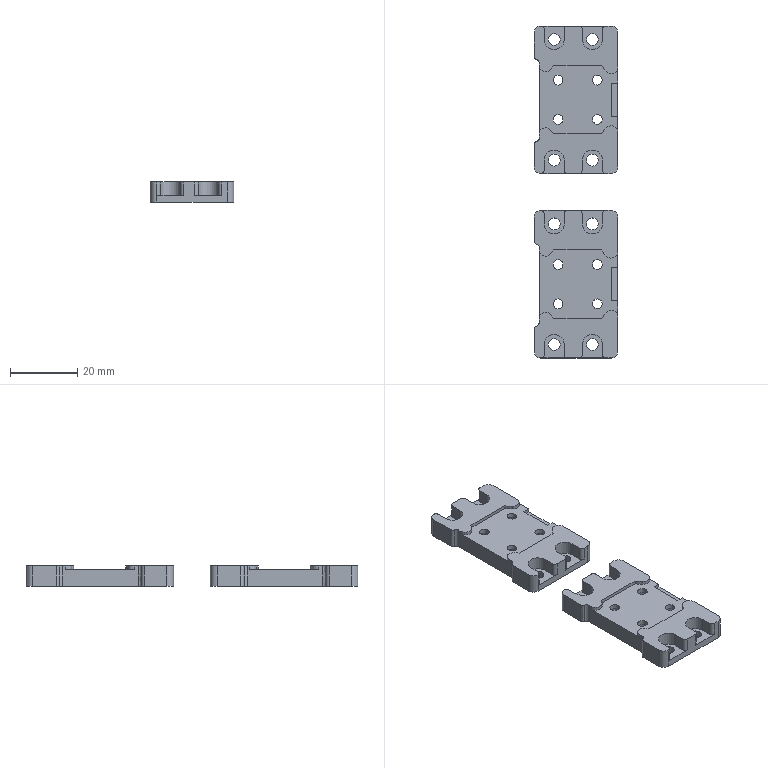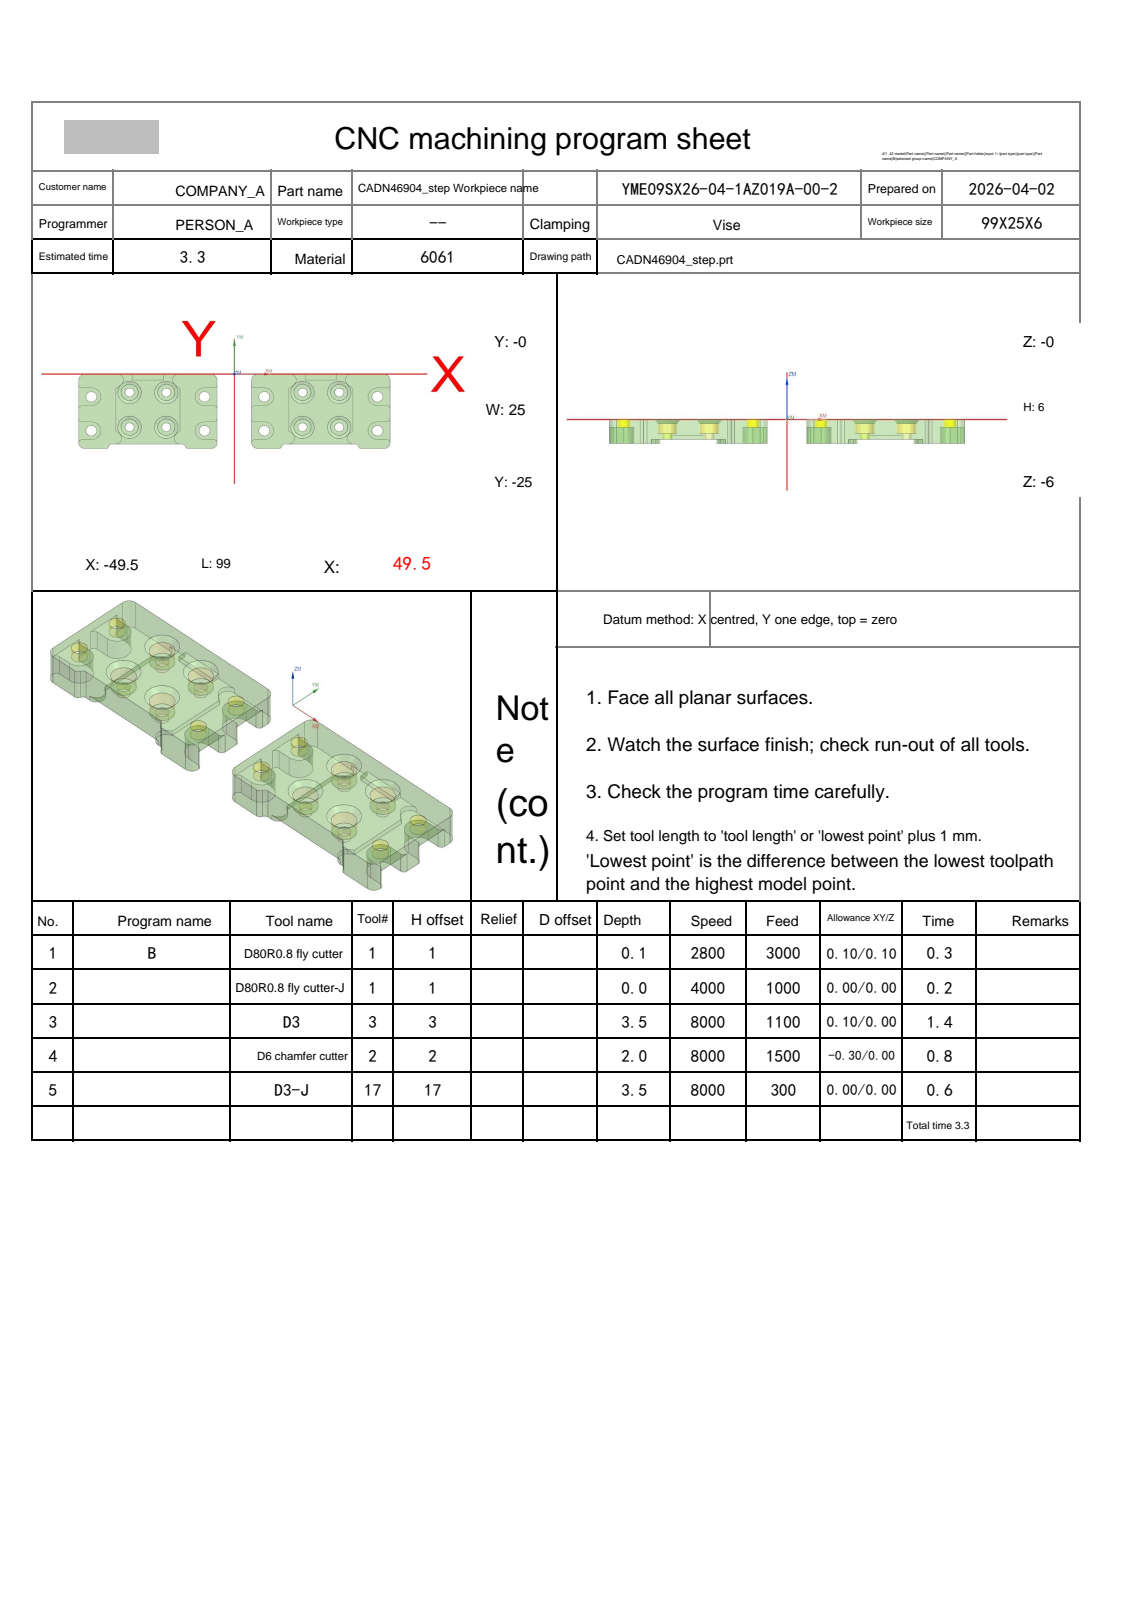NC program | NX | posted by the shop | part box 25 x 99 x 6 mm
Whole program:
%
O0001
(Machine time: 4.27 MIN)
(===Total Tool:4===)
(T1=D80R0.8 fly cutter D=80.  R=0.8  D-  H01 Z=0.    )
(T3=D3      D=3.   R=0.   D-  H03 Z=-3.5  )
(T2=D6 chamfer cutter   D=6.   R=0.   D-  H02 Z=-2.05 )
(T17=D3-J   D=3.   R=0.   D-  H17 Z=-3.5  )
G80 G90 G17 G49 G40
G91 G28 Z0
M01
N1 T01 M06
(D80R0.8 fly cutter  D=80. R=0.8 H=01 ce=0.10 di=0.10)
G00 G90 G54 X101.597 Y-10.58 M03 S2800
G43 H01 Z20.
M08
Z3.525
G01 Z1.525 F3000.
X89.597 Y-10.807
X-89.597 Y-14.193
X-101.597 Y-14.42
Z3.525
G00 X101.597 Y-10.58
Z3.05
G01 Z1.05
X89.597 Y-10.807
X-89.597 Y-14.193
X-101.597 Y-14.42
Z3.05
G00 X101.597 Y-10.58
Z2.575
G01 Z.575
X89.597 Y-10.807
X-89.597 Y-14.193
X-101.597 Y-14.42
Z2.575
G00 X101.597 Y-10.58
Z2.1
G01 Z.1
X89.597 Y-10.807
X-89.597 Y-14.193
X-101.597 Y-14.42
Z2.1
G00 Z20.
G91 G28 Z0.0
M05
M09
G91 G28 Z0.0
M01
N2 T01 M06
(D80R0.8 fly cutter-J  D=80. R=0.8 H=01 ce=0.00 di=0.00)
G00 G90 G54 X101.499 Y-10.584 M03 S4000
G43 H01 Z20.
M08
Z2.
G01 Z0.0 F1000.
X89.499 Y-10.81
X-89.499 Y-14.19
X-101.499 Y-14.416
Z2.
G00 Z20.
G91 G28 Z0.0
M05
M09
G91 G28 Z0.0
M01
N3 T03 M06
(D3  D=3. R=0. H=03 ce=0.10 di=0.00)
G00 G90 G54 X-21.671 Y-17.829 M03 S8000
G43 H03 Z20.
M08
Z1.3
G03 X-21.096 Y-17.254 I0.0 J.575 F1100.
X-21.671 Y-16.679 I-.575 J0.0
X-21.671 Y-16.679 Z1.1 I0.0 J-1.15
X-21.671 Y-16.679 Z.9 I0.0 J-1.15
X-21.671 Y-16.679 Z.7 I0.0 J-1.15
X-21.671 Y-16.679 Z.5 I0.0 J-1.15
X-21.671 Y-16.679 Z.3 I0.0 J-1.15
X-21.671 Y-16.679 Z.1 I0.0 J-1.15
X-21.671 Y-16.679 Z-.1 I0.0 J-1.15
X-21.671 Y-16.679 Z-.3 I0.0 J-1.15
X-21.671 Y-16.679 Z-.5 I0.0 J-1.15
X-21.671 Y-16.679 Z-.7 I0.0 J-1.15
X-21.671 Y-16.679 Z-.9 I0.0 J-1.15
X-21.671 Y-16.679 Z-1.1 I0.0 J-1.15
X-21.671 Y-16.679 Z-1.3 I0.0 J-1.15
X-21.671 Y-16.679 Z-1.5 I0.0 J-1.15
X-21.671 Y-16.679 Z-1.7 I0.0 J-1.15
X-21.671 Y-16.679 Z-1.9 I0.0 J-1.15
X-21.671 Y-16.679 Z-2.1 I0.0 J-1.15
X-21.671 Y-16.679 Z-2.3 I0.0 J-1.15
X-21.671 Y-16.679 Z-2.5 I0.0 J-1.15
X-21.671 Y-16.679 Z-2.7 I0.0 J-1.15
X-21.671 Y-16.679 Z-2.9 I0.0 J-1.15
X-21.671 Y-16.679 Z-3.1 I0.0 J-1.15
X-21.671 Y-16.679 Z-3.3 I0.0 J-1.15
X-21.671 Y-16.679 Z-3.5 I0.0 J-1.15
X-22.821 Y-17.829 I0.0 J-1.15
X-21.671 Y-18.979 I1.15 J0.0
X-20.521 Y-17.829 I0.0 J1.15
X-21.671 Y-16.679 I-1.15 J0.0
X-22.246 Y-17.254 I0.0 J-.575
X-21.671 Y-17.829 I.575 J0.0
G00 Z20.
X-33.329 Y-6.162
Z1.3
G03 X-32.754 Y-5.587 I0.0 J.575
X-33.329 Y-5.012 I-.575 J0.0
X-33.329 Y-5.012 Z1.1 I0.0 J-1.15
X-33.329 Y-5.012 Z.9 I0.0 J-1.15
X-33.329 Y-5.012 Z.7 I0.0 J-1.15
X-33.329 Y-5.012 Z.5 I0.0 J-1.15
X-33.329 Y-5.012 Z.3 I0.0 J-1.15
X-33.329 Y-5.012 Z.1 I0.0 J-1.15
X-33.329 Y-5.012 Z-.1 I0.0 J-1.15
X-33.329 Y-5.012 Z-.3 I0.0 J-1.15
X-33.329 Y-5.012 Z-.5 I0.0 J-1.15
X-33.329 Y-5.012 Z-.7 I0.0 J-1.15
X-33.329 Y-5.012 Z-.9 I0.0 J-1.15
X-33.329 Y-5.012 Z-1.1 I0.0 J-1.15
X-33.329 Y-5.012 Z-1.3 I0.0 J-1.15
X-33.329 Y-5.012 Z-1.5 I0.0 J-1.15
X-33.329 Y-5.012 Z-1.7 I0.0 J-1.15
X-33.329 Y-5.012 Z-1.9 I0.0 J-1.15
X-33.329 Y-5.012 Z-2.1 I0.0 J-1.15
X-33.329 Y-5.012 Z-2.3 I0.0 J-1.15
X-33.329 Y-5.012 Z-2.5 I0.0 J-1.15
X-33.329 Y-5.012 Z-2.7 I0.0 J-1.15
X-33.329 Y-5.012 Z-2.9 I0.0 J-1.15
X-33.329 Y-5.012 Z-3.1 I0.0 J-1.15
X-33.329 Y-5.012 Z-3.3 I0.0 J-1.15
X-33.329 Y-5.012 Z-3.5 I0.0 J-1.15
X-34.479 Y-6.162 I0.0 J-1.15
X-33.329 Y-7.312 I1.15 J0.0
X-32.179 Y-6.162 I0.0 J1.15
X-33.329 Y-5.012 I-1.15 J0.0
X-33.904 Y-5.587 I0.0 J-.575
X-33.329 Y-6.162 I.575 J0.0
G00 Z20.
X-21.662 Y-6.171
Z.3
G03 X-21.087 Y-5.596 I0.0 J.575
X-21.662 Y-5.021 I-.575 J0.0
X-21.662 Y-5.021 Z.1 I0.0 J-1.15
X-21.662 Y-5.021 Z-.1 I0.0 J-1.15
X-21.662 Y-5.021 Z-.3 I0.0 J-1.15
X-21.662 Y-5.021 Z-.5 I0.0 J-1.15
X-21.662 Y-5.021 Z-.7 I0.0 J-1.15
X-21.662 Y-5.021 Z-.9 I0.0 J-1.15
X-21.662 Y-5.021 Z-1.1 I0.0 J-1.15
X-21.662 Y-5.021 Z-1.3 I0.0 J-1.15
X-21.662 Y-5.021 Z-1.5 I0.0 J-1.15
X-21.662 Y-5.021 Z-1.7 I0.0 J-1.15
X-21.662 Y-5.021 Z-1.9 I0.0 J-1.15
X-21.662 Y-5.021 Z-2.1 I0.0 J-1.15
X-21.662 Y-5.021 Z-2.3 I0.0 J-1.15
X-21.662 Y-5.021 Z-2.5 I0.0 J-1.15
X-21.662 Y-5.021 Z-2.7 I0.0 J-1.15
X-21.662 Y-5.021 Z-2.9 I0.0 J-1.15
X-21.662 Y-5.021 Z-3.1 I0.0 J-1.15
X-21.662 Y-5.021 Z-3.3 I0.0 J-1.15
X-21.662 Y-5.021 Z-3.5 I0.0 J-1.15
X-22.812 Y-6.171 I0.0 J-1.15
X-21.662 Y-7.321 I1.15 J0.0
X-20.512 Y-6.171 I0.0 J1.15
X-21.662 Y-5.021 I-1.15 J0.0
X-22.237 Y-5.596 I0.0 J-.575
X-21.662 Y-6.171 I.575 J0.0
G00 Z20.
X21.671 Y-6.162
Z1.3
G03 X22.246 Y-5.587 I0.0 J.575
X21.671 Y-5.012 I-.575 J0.0
X21.671 Y-5.012 Z1.1 I0.0 J-1.15
X21.671 Y-5.012 Z.9 I0.0 J-1.15
X21.671 Y-5.012 Z.7 I0.0 J-1.15
X21.671 Y-5.012 Z.5 I0.0 J-1.15
X21.671 Y-5.012 Z.3 I0.0 J-1.15
X21.671 Y-5.012 Z.1 I0.0 J-1.15
X21.671 Y-5.012 Z-.1 I0.0 J-1.15
X21.671 Y-5.012 Z-.3 I0.0 J-1.15
X21.671 Y-5.012 Z-.5 I0.0 J-1.15
X21.671 Y-5.012 Z-.7 I0.0 J-1.15
X21.671 Y-5.012 Z-.9 I0.0 J-1.15
X21.671 Y-5.012 Z-1.1 I0.0 J-1.15
X21.671 Y-5.012 Z-1.3 I0.0 J-1.15
X21.671 Y-5.012 Z-1.5 I0.0 J-1.15
X21.671 Y-5.012 Z-1.7 I0.0 J-1.15
X21.671 Y-5.012 Z-1.9 I0.0 J-1.15
X21.671 Y-5.012 Z-2.1 I0.0 J-1.15
X21.671 Y-5.012 Z-2.3 I0.0 J-1.15
X21.671 Y-5.012 Z-2.5 I0.0 J-1.15
X21.671 Y-5.012 Z-2.7 I0.0 J-1.15
X21.671 Y-5.012 Z-2.9 I0.0 J-1.15
X21.671 Y-5.012 Z-3.1 I0.0 J-1.15
X21.671 Y-5.012 Z-3.3 I0.0 J-1.15
X21.671 Y-5.012 Z-3.5 I0.0 J-1.15
X20.521 Y-6.162 I0.0 J-1.15
X21.671 Y-7.312 I1.15 J0.0
X22.821 Y-6.162 I0.0 J1.15
X21.671 Y-5.012 I-1.15 J0.0
X21.096 Y-5.587 I0.0 J-.575
X21.671 Y-6.162 I.575 J0.0
G00 Z20.
X33.338 Y-6.171
Z1.3
G03 X33.913 Y-5.596 I0.0 J.575
X33.338 Y-5.021 I-.575 J0.0
X33.338 Y-5.021 Z1.1 I0.0 J-1.15
X33.338 Y-5.021 Z.9 I0.0 J-1.15
X33.338 Y-5.021 Z.7 I0.0 J-1.15
X33.338 Y-5.021 Z.5 I0.0 J-1.15
X33.338 Y-5.021 Z.3 I0.0 J-1.15
X33.338 Y-5.021 Z.1 I0.0 J-1.15
X33.338 Y-5.021 Z-.1 I0.0 J-1.15
X33.338 Y-5.021 Z-.3 I0.0 J-1.15
X33.338 Y-5.021 Z-.5 I0.0 J-1.15
X33.338 Y-5.021 Z-.7 I0.0 J-1.15
X33.338 Y-5.021 Z-.9 I0.0 J-1.15
X33.338 Y-5.021 Z-1.1 I0.0 J-1.15
X33.338 Y-5.021 Z-1.3 I0.0 J-1.15
X33.338 Y-5.021 Z-1.5 I0.0 J-1.15
X33.338 Y-5.021 Z-1.7 I0.0 J-1.15
X33.338 Y-5.021 Z-1.9 I0.0 J-1.15
X33.338 Y-5.021 Z-2.1 I0.0 J-1.15
X33.338 Y-5.021 Z-2.3 I0.0 J-1.15
X33.338 Y-5.021 Z-2.5 I0.0 J-1.15
X33.338 Y-5.021 Z-2.7 I0.0 J-1.15
X33.338 Y-5.021 Z-2.9 I0.0 J-1.15
X33.338 Y-5.021 Z-3.1 I0.0 J-1.15
X33.338 Y-5.021 Z-3.3 I0.0 J-1.15
X33.338 Y-5.021 Z-3.5 I0.0 J-1.15
X32.188 Y-6.171 I0.0 J-1.15
X33.338 Y-7.321 I1.15 J0.0
X34.488 Y-6.171 I0.0 J1.15
X33.338 Y-5.021 I-1.15 J0.0
X32.763 Y-5.596 I0.0 J-.575
X33.338 Y-6.171 I.575 J0.0
G00 Z20.
X33.329 Y-17.829
Z1.3
G03 X33.904 Y-17.254 I0.0 J.575
X33.329 Y-16.679 I-.575 J0.0
X33.329 Y-16.679 Z1.1 I0.0 J-1.15
X33.329 Y-16.679 Z.9 I0.0 J-1.15
X33.329 Y-16.679 Z.7 I0.0 J-1.15
X33.329 Y-16.679 Z.5 I0.0 J-1.15
X33.329 Y-16.679 Z.3 I0.0 J-1.15
X33.329 Y-16.679 Z.1 I0.0 J-1.15
X33.329 Y-16.679 Z-.1 I0.0 J-1.15
X33.329 Y-16.679 Z-.3 I0.0 J-1.15
X33.329 Y-16.679 Z-.5 I0.0 J-1.15
X33.329 Y-16.679 Z-.7 I0.0 J-1.15
X33.329 Y-16.679 Z-.9 I0.0 J-1.15
X33.329 Y-16.679 Z-1.1 I0.0 J-1.15
X33.329 Y-16.679 Z-1.3 I0.0 J-1.15
X33.329 Y-16.679 Z-1.5 I0.0 J-1.15
X33.329 Y-16.679 Z-1.7 I0.0 J-1.15
X33.329 Y-16.679 Z-1.9 I0.0 J-1.15
X33.329 Y-16.679 Z-2.1 I0.0 J-1.15
X33.329 Y-16.679 Z-2.3 I0.0 J-1.15
X33.329 Y-16.679 Z-2.5 I0.0 J-1.15
X33.329 Y-16.679 Z-2.7 I0.0 J-1.15
X33.329 Y-16.679 Z-2.9 I0.0 J-1.15
X33.329 Y-16.679 Z-3.1 I0.0 J-1.15
X33.329 Y-16.679 Z-3.3 I0.0 J-1.15
X33.329 Y-16.679 Z-3.5 I0.0 J-1.15
X32.179 Y-17.829 I0.0 J-1.15
X33.329 Y-18.979 I1.15 J0.0
X34.479 Y-17.829 I0.0 J1.15
X33.329 Y-16.679 I-1.15 J0.0
X32.754 Y-17.254 I0.0 J-.575
X33.329 Y-17.829 I.575 J0.0
G00 Z20.
G00 G90 X-33.338 Y-17.829 M03 S8000
Z20.
Z1.3
G03 X-32.763 Y-17.254 I0.0 J.575 F1100.
X-33.338 Y-16.679 I-.575 J0.0
X-33.338 Y-16.679 Z1.1 I0.0 J-1.15
X-33.338 Y-16.679 Z.9 I0.0 J-1.15
X-33.338 Y-16.679 Z.7 I0.0 J-1.15
X-33.338 Y-16.679 Z.5 I0.0 J-1.15
X-33.338 Y-16.679 Z.3 I0.0 J-1.15
X-33.338 Y-16.679 Z.1 I0.0 J-1.15
X-33.338 Y-16.679 Z-.1 I0.0 J-1.15
X-33.338 Y-16.679 Z-.3 I0.0 J-1.15
X-33.338 Y-16.679 Z-.5 I0.0 J-1.15
X-33.338 Y-16.679 Z-.7 I0.0 J-1.15
X-33.338 Y-16.679 Z-.9 I0.0 J-1.15
X-33.338 Y-16.679 Z-1.1 I0.0 J-1.15
X-33.338 Y-16.679 Z-1.3 I0.0 J-1.15
X-33.338 Y-16.679 Z-1.5 I0.0 J-1.15
X-33.338 Y-16.679 Z-1.7 I0.0 J-1.15
X-33.338 Y-16.679 Z-1.9 I0.0 J-1.15
X-33.338 Y-16.679 Z-2.1 I0.0 J-1.15
X-33.338 Y-16.679 Z-2.3 I0.0 J-1.15
X-33.338 Y-16.679 Z-2.5 I0.0 J-1.15
X-33.338 Y-16.679 Z-2.7 I0.0 J-1.15
X-33.338 Y-16.679 Z-2.9 I0.0 J-1.15
X-33.338 Y-16.679 Z-3.1 I0.0 J-1.15
X-33.338 Y-16.679 Z-3.3 I0.0 J-1.15
X-33.338 Y-16.679 Z-3.5 I0.0 J-1.15
X-34.488 Y-17.829 I0.0 J-1.15
X-33.338 Y-18.979 I1.15 J0.0
X-32.188 Y-17.829 I0.0 J1.15
X-33.338 Y-16.679 I-1.15 J0.0
X-33.913 Y-17.254 I0.0 J-.575
X-33.338 Y-17.829 I.575 J0.0
G00 Z20.
X21.662
Z1.3
G03 X22.237 Y-17.254 I0.0 J.575
X21.662 Y-16.679 I-.575 J0.0
X21.662 Y-16.679 Z1.1 I0.0 J-1.15
X21.662 Y-16.679 Z.9 I0.0 J-1.15
X21.662 Y-16.679 Z.7 I0.0 J-1.15
X21.662 Y-16.679 Z.5 I0.0 J-1.15
X21.662 Y-16.679 Z.3 I0.0 J-1.15
X21.662 Y-16.679 Z.1 I0.0 J-1.15
X21.662 Y-16.679 Z-.1 I0.0 J-1.15
X21.662 Y-16.679 Z-.3 I0.0 J-1.15
X21.662 Y-16.679 Z-.5 I0.0 J-1.15
X21.662 Y-16.679 Z-.7 I0.0 J-1.15
X21.662 Y-16.679 Z-.9 I0.0 J-1.15
X21.662 Y-16.679 Z-1.1 I0.0 J-1.15
X21.662 Y-16.679 Z-1.3 I0.0 J-1.15
X21.662 Y-16.679 Z-1.5 I0.0 J-1.15
X21.662 Y-16.679 Z-1.7 I0.0 J-1.15
X21.662 Y-16.679 Z-1.9 I0.0 J-1.15
X21.662 Y-16.679 Z-2.1 I0.0 J-1.15
X21.662 Y-16.679 Z-2.3 I0.0 J-1.15
X21.662 Y-16.679 Z-2.5 I0.0 J-1.15
X21.662 Y-16.679 Z-2.7 I0.0 J-1.15
X21.662 Y-16.679 Z-2.9 I0.0 J-1.15
X21.662 Y-16.679 Z-3.1 I0.0 J-1.15
X21.662 Y-16.679 Z-3.3 I0.0 J-1.15
X21.662 Y-16.679 Z-3.5 I0.0 J-1.15
X20.512 Y-17.829 I0.0 J-1.15
X21.662 Y-18.979 I1.15 J0.0
X22.812 Y-17.829 I0.0 J1.15
X21.662 Y-16.679 I-1.15 J0.0
X21.087 Y-17.254 I0.0 J-.575
X21.662 Y-17.829 I.575 J0.0
G00 Z20.
G91 G28 Z0.0
M05
M09
G91 G28 Z0.0
M01
N4 T02 M06
(D6 chamfer cutter  D=6. R=0. H=02 ce=0.00 di=0.00)
G00 G90 G54 X-45.5 Y-7.619 M03 S8000
G43 H02 Z20.
M08
G98 G81 X-45.5 Y-7.619 Z-2.05 R3. F1000.
Y-19.
X-9.5
Y-7.619
X9.5
Y-19.
X45.5
Y-7.619
G80
G00 Z20.
G00 G90 X-35.545 Y-5.783 M03 S7000
Z20.
Z2.5
G01 X-35.572 Y-5.944 Z2.441 F500.
X-35.58 Y-6.264 Z2.324
X-35.543 Y-6.582 Z2.207
X-35.461 Y-6.892 Z2.091
X-35.336 Y-7.187 Z1.974
X-35.22 Y-7.388 Z1.89
X-35.027 Y-7.643 Z1.773
X-34.8 Y-7.869 Z1.657
X-34.543 Y-8.06 Z1.54
X-34.262 Y-8.213 Z1.424
X-33.962 Y-8.325 Z1.307
X-33.649 Y-8.392 Z1.191
X-33.329 Y-8.415 Z1.074
X-33.01 Y-8.392 Z.958
X-32.697 Y-8.325 Z.841
X-32.397 Y-8.213 Z.724
X-32.116 Y-8.06 Z.608
X-31.859 Y-7.869 Z.491
X-31.632 Y-7.643 Z.375
X-31.439 Y-7.388 Z.258
X-31.323 Y-7.187 Z.174
X-31.198 Y-6.892 Z.057
X-31.116 Y-6.582 Z-.059
X-31.079 Y-6.264 Z-.176
X-31.087 Y-5.944 Z-.292
X-31.141 Y-5.629 Z-.409
X-31.238 Y-5.324 Z-.525
X-31.378 Y-5.036 Z-.642
X-31.558 Y-4.771 Z-.759
X-31.773 Y-4.533 Z-.875
X-32.019 Y-4.329 Z-.992
X-32.293 Y-4.162 Z-1.108
X-32.587 Y-4.035 Z-1.225
X-32.895 Y-3.951 Z-1.341
X-33.213 Y-3.912 Z-1.458
X-33.329 Z-1.5
G03 X-35.579 Y-6.162 I0.0 J-2.25
X-33.329 Y-8.412 I2.25 J0.0
X-31.079 Y-6.162 I0.0 J2.25
X-33.329 Y-3.912 I-2.25 J0.0
X-33.825 Y-3.968 I0.0 J-2.25
G01 Z1.
G00 Z20.
X-35.553 Y-17.45
Z2.5
G01 X-35.58 Y-17.611 Z2.441
X-35.588 Y-17.932 Z2.324
X-35.551 Y-18.25 Z2.207
X-35.469 Y-18.559 Z2.091
X-35.344 Y-18.854 Z1.974
X-35.228 Y-19.055 Z1.89
X-35.035 Y-19.311 Z1.773
X-34.808 Y-19.536 Z1.657
X-34.551 Y-19.728 Z1.54
X-34.27 Y-19.88 Z1.424
X-33.97 Y-19.992 Z1.307
X-33.657 Y-20.06 Z1.191
X-33.338 Y-20.082 Z1.074
X-33.018 Y-20.06 Z.958
X-32.706 Y-19.992 Z.841
X-32.405 Y-19.88 Z.724
X-32.124 Y-19.728 Z.608
X-31.867 Y-19.536 Z.491
X-31.64 Y-19.311 Z.375
X-31.447 Y-19.055 Z.258
X-31.331 Y-18.854 Z.174
X-31.206 Y-18.559 Z.057
X-31.124 Y-18.25 Z-.059
X-31.087 Y-17.932 Z-.176
X-31.095 Y-17.611 Z-.292
X-31.149 Y-17.296 Z-.409
X-31.247 Y-16.991 Z-.525
X-31.387 Y-16.703 Z-.642
X-31.566 Y-16.438 Z-.759
X-31.781 Y-16.201 Z-.875
X-32.028 Y-15.996 Z-.992
X-32.301 Y-15.829 Z-1.108
X-32.595 Y-15.703 Z-1.225
X-32.904 Y-15.619 Z-1.341
X-33.222 Y-15.579 Z-1.458
X-33.338 Z-1.5
G03 X-35.588 Y-17.829 I0.0 J-2.25
X-33.338 Y-20.079 I2.25 J0.0
X-31.088 Y-17.829 I0.0 J2.25
X-33.338 Y-15.579 I-2.25 J0.0
X-33.834 Y-15.635 I0.0 J-2.25
G01 Z1.
G00 Z20.
X-23.886 Y-17.45
Z2.5
G01 X-23.913 Y-17.611 Z2.441
X-23.921 Y-17.932 Z2.324
X-23.884 Y-18.25 Z2.207
X-23.802 Y-18.559 Z2.091
X-23.677 Y-18.854 Z1.974
X-23.561 Y-19.055 Z1.89
X-23.368 Y-19.311 Z1.773
X-23.141 Y-19.536 Z1.657
X-22.884 Y-19.728 Z1.54
X-22.603 Y-19.88 Z1.424
X-22.303 Y-19.992 Z1.307
X-21.99 Y-20.06 Z1.191
X-21.671 Y-20.082 Z1.074
X-21.351 Y-20.06 Z.958
X-21.038 Y-19.992 Z.841
X-20.738 Y-19.88 Z.724
X-20.457 Y-19.728 Z.608
X-20.2 Y-19.536 Z.491
X-19.973 Y-19.311 Z.375
X-19.78 Y-19.055 Z.258
X-19.664 Y-18.854 Z.174
X-19.539 Y-18.559 Z.057
X-19.457 Y-18.25 Z-.059
X-19.42 Y-17.932 Z-.176
X-19.428 Y-17.611 Z-.292
X-19.482 Y-17.296 Z-.409
X-19.579 Y-16.991 Z-.525
X-19.719 Y-16.703 Z-.642
X-19.899 Y-16.438 Z-.759
X-20.114 Y-16.201 Z-.875
X-20.36 Y-15.996 Z-.992
X-20.634 Y-15.829 Z-1.108
X-20.928 Y-15.703 Z-1.225
X-21.237 Y-15.619 Z-1.341
X-21.554 Y-15.579 Z-1.458
X-21.671 Z-1.5
G03 X-23.921 Y-17.829 I0.0 J-2.25
X-21.671 Y-20.079 I2.25 J0.0
X-19.421 Y-17.829 I0.0 J2.25
X-21.671 Y-15.579 I-2.25 J0.0
X-22.166 Y-15.635 I0.0 J-2.25
G01 Z1.
G00 Z20.
X-23.877 Y-5.791
Z2.5
G01 X-23.905 Y-5.952 Z2.441
X-23.913 Y-6.273 Z2.324
X-23.876 Y-6.591 Z2.207
X-23.794 Y-6.9 Z2.091
X-23.669 Y-7.195 Z1.974
X-23.553 Y-7.396 Z1.89
X-23.36 Y-7.652 Z1.773
X-23.133 Y-7.877 Z1.657
X-22.876 Y-8.069 Z1.54
X-22.595 Y-8.222 Z1.424
X-22.294 Y-8.333 Z1.307
X-21.982 Y-8.401 Z1.191
X-21.662 Y-8.424 Z1.074
X-21.343 Y-8.401 Z.958
X-21.03 Y-8.333 Z.841
X-20.73 Y-8.222 Z.724
X-20.449 Y-8.069 Z.608
X-20.192 Y-7.877 Z.491
X-19.965 Y-7.652 Z.375
X-19.772 Y-7.396 Z.258
X-19.656 Y-7.195 Z.174
X-19.531 Y-6.9 Z.057
X-19.449 Y-6.591 Z-.059
X-19.412 Y-6.273 Z-.176
X-19.42 Y-5.952 Z-.292
X-19.473 Y-5.637 Z-.409
X-19.571 Y-5.332 Z-.525
X-19.711 Y-5.044 Z-.642
X-19.89 Y-4.779 Z-.759
X-20.106 Y-4.542 Z-.875
X-20.352 Y-4.338 Z-.992
X-20.625 Y-4.17 Z-1.108
X-20.919 Y-4.044 Z-1.225
X-21.228 Y-3.96 Z-1.341
X-21.546 Y-3.921 Z-1.458
X-21.662 Z-1.5
G03 X-23.912 Y-6.171 I0.0 J-2.25
X-21.662 Y-8.421 I2.25 J0.0
X-19.412 Y-6.171 I0.0 J2.25
X-21.662 Y-3.921 I-2.25 J0.0
X-22.158 Y-3.976 I0.0 J-2.25
G01 Z1.
G00 Z20.
X19.455 Y-5.783
Z2.5
G01 X19.428 Y-5.944 Z2.441
X19.42 Y-6.264 Z2.324
X19.457 Y-6.582 Z2.207
X19.539 Y-6.892 Z2.091
X19.664 Y-7.187 Z1.974
X19.78 Y-7.388 Z1.89
X19.973 Y-7.643 Z1.773
X20.2 Y-7.869 Z1.657
X20.457 Y-8.06 Z1.54
X20.738 Y-8.213 Z1.424
X21.038 Y-8.325 Z1.307
X21.351 Y-8.392 Z1.191
X21.671 Y-8.415 Z1.074
X21.99 Y-8.392 Z.958
X22.303 Y-8.325 Z.841
X22.603 Y-8.213 Z.724
X22.884 Y-8.06 Z.608
X23.141 Y-7.869 Z.491
X23.368 Y-7.643 Z.375
X23.561 Y-7.388 Z.258
X23.677 Y-7.187 Z.174
X23.802 Y-6.892 Z.057
X23.884 Y-6.582 Z-.059
X23.921 Y-6.264 Z-.176
X23.913 Y-5.944 Z-.292
X23.859 Y-5.629 Z-.409
X23.762 Y-5.324 Z-.525
X23.622 Y-5.036 Z-.642
X23.442 Y-4.771 Z-.759
X23.227 Y-4.533 Z-.875
X22.981 Y-4.329 Z-.992
X22.707 Y-4.162 Z-1.108
X22.413 Y-4.035 Z-1.225
X22.105 Y-3.951 Z-1.341
X21.787 Y-3.912 Z-1.458
X21.671 Z-1.5
G03 X19.421 Y-6.162 I0.0 J-2.25
X21.671 Y-8.412 I2.25 J0.0
X23.921 Y-6.162 I0.0 J2.25
X21.671 Y-3.912 I-2.25 J0.0
X21.175 Y-3.968 I0.0 J-2.25
G01 Z1.
G00 Z20.
X31.123 Y-5.791
Z2.5
G01 X31.095 Y-5.952 Z2.441
X31.087 Y-6.273 Z2.324
X31.124 Y-6.591 Z2.207
X31.206 Y-6.9 Z2.091
X31.331 Y-7.195 Z1.974
X31.447 Y-7.396 Z1.89
X31.64 Y-7.652 Z1.773
X31.867 Y-7.877 Z1.657
X32.124 Y-8.069 Z1.54
X32.405 Y-8.222 Z1.424
X32.706 Y-8.333 Z1.307
X33.018 Y-8.401 Z1.191
X33.338 Y-8.424 Z1.074
X33.657 Y-8.401 Z.958
X33.97 Y-8.333 Z.841
X34.27 Y-8.222 Z.724
X34.551 Y-8.069 Z.608
X34.808 Y-7.877 Z.491
X35.035 Y-7.652 Z.375
X35.228 Y-7.396 Z.258
X35.344 Y-7.195 Z.174
X35.469 Y-6.9 Z.057
X35.551 Y-6.591 Z-.059
X35.588 Y-6.273 Z-.176
X35.58 Y-5.952 Z-.292
X35.527 Y-5.637 Z-.409
X35.429 Y-5.332 Z-.525
X35.289 Y-5.044 Z-.642
X35.11 Y-4.779 Z-.759
X34.894 Y-4.542 Z-.875
X34.648 Y-4.338 Z-.992
X34.375 Y-4.17 Z-1.108
X34.081 Y-4.044 Z-1.225
X33.772 Y-3.96 Z-1.341
X33.454 Y-3.921 Z-1.458
X33.338 Z-1.5
G03 X31.088 Y-6.171 I0.0 J-2.25
X33.338 Y-8.421 I2.25 J0.0
X35.588 Y-6.171 I0.0 J2.25
X33.338 Y-3.921 I-2.25 J0.0
X32.842 Y-3.976 I0.0 J-2.25
G01 Z1.
G00 Z20.
X31.114 Y-17.45
Z2.5
G01 X31.087 Y-17.611 Z2.441
X31.079 Y-17.932 Z2.324
X31.116 Y-18.25 Z2.207
X31.198 Y-18.559 Z2.091
X31.323 Y-18.854 Z1.974
X31.439 Y-19.055 Z1.89
X31.632 Y-19.311 Z1.773
X31.859 Y-19.536 Z1.657
X32.116 Y-19.728 Z1.54
X32.397 Y-19.88 Z1.424
X32.697 Y-19.992 Z1.307
X33.01 Y-20.06 Z1.191
X33.329 Y-20.082 Z1.074
X33.649 Y-20.06 Z.958
X33.962 Y-19.992 Z.841
X34.262 Y-19.88 Z.724
X34.543 Y-19.728 Z.608
X34.8 Y-19.536 Z.491
X35.027 Y-19.311 Z.375
X35.22 Y-19.055 Z.258
X35.336 Y-18.854 Z.174
X35.461 Y-18.559 Z.057
X35.543 Y-18.25 Z-.059
X35.58 Y-17.932 Z-.176
X35.572 Y-17.611 Z-.292
X35.518 Y-17.296 Z-.409
X35.421 Y-16.991 Z-.525
X35.281 Y-16.703 Z-.642
X35.101 Y-16.438 Z-.759
X34.886 Y-16.201 Z-.875
X34.64 Y-15.996 Z-.992
X34.366 Y-15.829 Z-1.108
X34.072 Y-15.703 Z-1.225
X33.763 Y-15.619 Z-1.341
X33.446 Y-15.579 Z-1.458
X33.329 Z-1.5
G03 X31.079 Y-17.829 I0.0 J-2.25
X33.329 Y-20.079 I2.25 J0.0
X35.579 Y-17.829 I0.0 J2.25
X33.329 Y-15.579 I-2.25 J0.0
X32.834 Y-15.635 I0.0 J-2.25
G01 Z1.
G00 Z20.
X19.447 Y-17.45
Z2.5
G01 X19.42 Y-17.611 Z2.441
X19.412 Y-17.932 Z2.324
X19.449 Y-18.25 Z2.207
X19.531 Y-18.559 Z2.091
X19.656 Y-18.854 Z1.974
X19.772 Y-19.055 Z1.89
X19.965 Y-19.311 Z1.773
X20.192 Y-19.536 Z1.657
X20.449 Y-19.728 Z1.54
X20.73 Y-19.88 Z1.424
X21.03 Y-19.992 Z1.307
X21.343 Y-20.06 Z1.191
X21.662 Y-20.082 Z1.074
X21.982 Y-20.06 Z.958
X22.294 Y-19.992 Z.841
X22.595 Y-19.88 Z.724
X22.876 Y-19.728 Z.608
X23.133 Y-19.536 Z.491
X23.36 Y-19.311 Z.375
X23.553 Y-19.055 Z.258
X23.669 Y-18.854 Z.174
X23.794 Y-18.559 Z.057
X23.876 Y-18.25 Z-.059
X23.913 Y-17.932 Z-.176
X23.905 Y-17.611 Z-.292
X23.851 Y-17.296 Z-.409
X23.753 Y-16.991 Z-.525
X23.613 Y-16.703 Z-.642
X23.434 Y-16.438 Z-.759
X23.219 Y-16.201 Z-.875
X22.972 Y-15.996 Z-.992
X22.699 Y-15.829 Z-1.108
X22.405 Y-15.703 Z-1.225
X22.096 Y-15.619 Z-1.341
X21.778 Y-15.579 Z-1.458
X21.662 Z-1.5
G03 X19.412 Y-17.829 I0.0 J-2.25
X21.662 Y-20.079 I2.25 J0.0
X23.912 Y-17.829 I0.0 J2.25
X21.662 Y-15.579 I-2.25 J0.0
X21.166 Y-15.635 I0.0 J-2.25
G01 Z1.
G00 Z20.
G00 G90 X25.616 Y-24.2 M03 S7000
Z20.
Z2.5
G01 X16. Z-1. F1500.
G03 X15.71 Y-24.425 I0.0 J-.3
G02 X14.064 Y-25.7 I-1.646 J.425
G01 X7.5
G02 X4.8 Y-23. I0.0 J2.7
G01 Y-2.
G02 X7.5 Y.7 I2.7 J0.0
G01 X47.5
G02 X50.2 Y-2. I0.0 J-2.7
G01 Y-23.
G02 X47.5 Y-25.7 I-2.7 J0.0
G01 X40.436
G02 X38.79 Y-24.425 I0.0 J1.7
G03 X38.5 Y-24.2 I-.29 J-.075
G01 X16.
G03 X15.71 Y-24.425 I0.0 J-.3
G01 X15.699 Y-24.476
X15.68 Y-24.525
Z1.5
G00 Z20.
X-29.384 Y-24.2
Z2.5
G01 X-39. Z-1.
G03 X-39.29 Y-24.425 I0.0 J-.3
G02 X-40.936 Y-25.7 I-1.646 J.425
G01 X-47.5
G02 X-50.2 Y-23. I0.0 J2.7
G01 Y-2.
G02 X-47.5 Y.7 I2.7 J0.0
G01 X-7.5
G02 X-4.8 Y-2. I0.0 J-2.7
G01 Y-23.
G02 X-7.5 Y-25.7 I-2.7 J0.0
G01 X-14.564
G02 X-16.21 Y-24.425 I0.0 J1.7
G03 X-16.5 Y-24.2 I-.29 J-.075
G01 X-39.
G03 X-39.29 Y-24.425 I0.0 J-.3
G01 X-39.301 Y-24.476
X-39.32 Y-24.525
Z1.5
G00 Z20.
G91 G28 Z0.0
M05
M09
G91 G28 Z0.0
M01
N5 T17 M06
(D3-J  D=3. R=0. H=17 ce=0.00 di=0.00)
G00 G90 G54 X-21.671 Y-17.829 M03 S8000
G43 H17 Z20.
M08
Z-1.
G01 X-21.358 Y-17.039 F300.
X-21.335 Y-16.915
G03 X-21.671 Y-16.579 I-.336 J0.0
X-22.921 Y-17.829 I0.0 J-1.25
X-21.671 Y-19.079 I1.25 J0.0
X-20.421 Y-17.829 I0.0 J1.25
X-21.671 Y-16.579 I-1.25 J0.0
X-22.157 Y-16.678 I0.0 J-1.25
X-22.362 Y-16.988 I.131 J-.309
X-22.266 Y-17.223 I.336 J0.0
G01 X-21.671 Y-17.829
Z-3.5 F10000.
X-21.358 Y-17.039 F300.
X-21.335 Y-16.915
G03 X-21.671 Y-16.579 I-.336 J0.0
X-22.921 Y-17.829 I0.0 J-1.25
X-21.671 Y-19.079 I1.25 J0.0
X-20.421 Y-17.829 I0.0 J1.25
X-21.671 Y-16.579 I-1.25 J0.0
X-22.157 Y-16.678 I0.0 J-1.25
X-22.362 Y-16.988 I.131 J-.309
X-22.266 Y-17.223 I.336 J0.0
G01 X-21.671 Y-17.829
G00 Z20.
X-33.329 Y-6.162
Z-1.
G01 X-33.017 Y-5.372
X-32.993 Y-5.248
G03 X-33.329 Y-4.912 I-.336 J0.0
X-34.579 Y-6.162 I0.0 J-1.25
X-33.329 Y-7.412 I1.25 J0.0
X-32.079 Y-6.162 I0.0 J1.25
X-33.329 Y-4.912 I-1.25 J0.0
X-33.816 Y-5.011 I0.0 J-1.25
X-34.021 Y-5.32 I.131 J-.309
X-33.925 Y-5.556 I.336 J0.0
G01 X-33.329 Y-6.162
Z-3.5 F10000.
X-33.017 Y-5.372 F300.
X-32.993 Y-5.248
G03 X-33.329 Y-4.912 I-.336 J0.0
X-34.579 Y-6.162 I0.0 J-1.25
X-33.329 Y-7.412 I1.25 J0.0
X-32.079 Y-6.162 I0.0 J1.25
X-33.329 Y-4.912 I-1.25 J0.0
X-33.816 Y-5.011 I0.0 J-1.25
X-34.021 Y-5.32 I.131 J-.309
X-33.925 Y-5.556 I.336 J0.0
G01 X-33.329 Y-6.162
G00 Z20.
X-21.662 Y-6.171
Z-3.5
G01 X-21.35 Y-5.38
X-21.326 Y-5.257
G03 X-21.662 Y-4.921 I-.336 J0.0
X-22.912 Y-6.171 I0.0 J-1.25
X-21.662 Y-7.421 I1.25 J0.0
X-20.412 Y-6.171 I0.0 J1.25
X-21.662 Y-4.921 I-1.25 J0.0
X-22.149 Y-5.019 I0.0 J-1.25
X-22.354 Y-5.329 I.131 J-.309
X-22.258 Y-5.564 I.336 J0.0
G01 X-21.662 Y-6.171
G00 Z20.
X21.671 Y-6.162
Z-1.
G01 X21.983 Y-5.372
X22.007 Y-5.248
G03 X21.671 Y-4.912 I-.336 J0.0
X20.421 Y-6.162 I0.0 J-1.25
X21.671 Y-7.412 I1.25 J0.0
X22.921 Y-6.162 I0.0 J1.25
X21.671 Y-4.912 I-1.25 J0.0
X21.184 Y-5.011 I0.0 J-1.25
X20.979 Y-5.32 I.131 J-.309
X21.075 Y-5.556 I.336 J0.0
G01 X21.671 Y-6.162
Z-3.5 F10000.
X21.983 Y-5.372 F300.
X22.007 Y-5.248
G03 X21.671 Y-4.912 I-.336 J0.0
X20.421 Y-6.162 I0.0 J-1.25
X21.671 Y-7.412 I1.25 J0.0
X22.921 Y-6.162 I0.0 J1.25
X21.671 Y-4.912 I-1.25 J0.0
X21.184 Y-5.011 I0.0 J-1.25
X20.979 Y-5.32 I.131 J-.309
X21.075 Y-5.556 I.336 J0.0
G01 X21.671 Y-6.162
G00 Z20.
X33.338 Y-6.171
Z-1.
G01 X33.65 Y-5.38
X33.674 Y-5.257
G03 X33.338 Y-4.921 I-.336 J0.0
X32.088 Y-6.171 I0.0 J-1.25
X33.338 Y-7.421 I1.25 J0.0
X34.588 Y-6.171 I0.0 J1.25
X33.338 Y-4.921 I-1.25 J0.0
X32.851 Y-5.019 I0.0 J-1.25
X32.646 Y-5.329 I.131 J-.309
X32.742 Y-5.564 I.336 J0.0
G01 X33.338 Y-6.171
Z-3.5 F10000.
X33.65 Y-5.38 F300.
X33.674 Y-5.257
G03 X33.338 Y-4.921 I-.336 J0.0
X32.088 Y-6.171 I0.0 J-1.25
X33.338 Y-7.421 I1.25 J0.0
X34.588 Y-6.171 I0.0 J1.25
X33.338 Y-4.921 I-1.25 J0.0
X32.851 Y-5.019 I0.0 J-1.25
X32.646 Y-5.329 I.131 J-.309
X32.742 Y-5.564 I.336 J0.0
G01 X33.338 Y-6.171
G00 Z20.
X33.329 Y-17.829
Z-1.
G01 X33.642 Y-17.039
X33.665 Y-16.915
G03 X33.329 Y-16.579 I-.336 J0.0
X32.079 Y-17.829 I0.0 J-1.25
X33.329 Y-19.079 I1.25 J0.0
X34.579 Y-17.829 I0.0 J1.25
X33.329 Y-16.579 I-1.25 J0.0
X32.843 Y-16.678 I0.0 J-1.25
X32.638 Y-16.988 I.131 J-.309
X32.734 Y-17.223 I.336 J0.0
G01 X33.329 Y-17.829
Z-3.5 F10000.
X33.642 Y-17.039 F300.
X33.665 Y-16.915
G03 X33.329 Y-16.579 I-.336 J0.0
X32.079 Y-17.829 I0.0 J-1.25
X33.329 Y-19.079 I1.25 J0.0
X34.579 Y-17.829 I0.0 J1.25
X33.329 Y-16.579 I-1.25 J0.0
X32.843 Y-16.678 I0.0 J-1.25
X32.638 Y-16.988 I.131 J-.309
X32.734 Y-17.223 I.336 J0.0
G01 X33.329 Y-17.829
G00 Z20.
G00 G90 X-33.338 Y-17.829 M03 S8000
Z20.
Z-1.
G01 X-33.025 Y-17.039 F300.
X-33.002 Y-16.915
G03 X-33.338 Y-16.579 I-.336 J0.0
X-34.588 Y-17.829 I0.0 J-1.25
X-33.338 Y-19.079 I1.25 J0.0
X-32.088 Y-17.829 I0.0 J1.25
X-33.338 Y-16.579 I-1.25 J0.0
X-33.825 Y-16.678 I0.0 J-1.25
X-34.03 Y-16.988 I.131 J-.309
X-33.933 Y-17.223 I.336 J0.0
G01 X-33.338 Y-17.829
Z-3.5 F10000.
X-33.025 Y-17.039 F300.
X-33.002 Y-16.915
G03 X-33.338 Y-16.579 I-.336 J0.0
X-34.588 Y-17.829 I0.0 J-1.25
X-33.338 Y-19.079 I1.25 J0.0
X-32.088 Y-17.829 I0.0 J1.25
X-33.338 Y-16.579 I-1.25 J0.0
X-33.825 Y-16.678 I0.0 J-1.25
X-34.03 Y-16.988 I.131 J-.309
X-33.933 Y-17.223 I.336 J0.0
G01 X-33.338 Y-17.829
G00 Z20.
X21.662
Z-1.
G01 X21.975 Y-17.039
X21.998 Y-16.915
G03 X21.662 Y-16.579 I-.336 J0.0
X20.412 Y-17.829 I0.0 J-1.25
X21.662 Y-19.079 I1.25 J0.0
X22.912 Y-17.829 I0.0 J1.25
X21.662 Y-16.579 I-1.25 J0.0
X21.175 Y-16.678 I0.0 J-1.25
X20.97 Y-16.988 I.131 J-.309
X21.067 Y-17.223 I.336 J0.0
G01 X21.662 Y-17.829
Z-3.5 F10000.
X21.975 Y-17.039 F300.
X21.998 Y-16.915
G03 X21.662 Y-16.579 I-.336 J0.0
X20.412 Y-17.829 I0.0 J-1.25
X21.662 Y-19.079 I1.25 J0.0
X22.912 Y-17.829 I0.0 J1.25
X21.662 Y-16.579 I-1.25 J0.0
X21.175 Y-16.678 I0.0 J-1.25
X20.97 Y-16.988 I.131 J-.309
X21.067 Y-17.223 I.336 J0.0
G01 X21.662 Y-17.829
G00 Z20.
M05
M09
G91 G28 Z0.0
G91 G28 Y0.0
M30
%